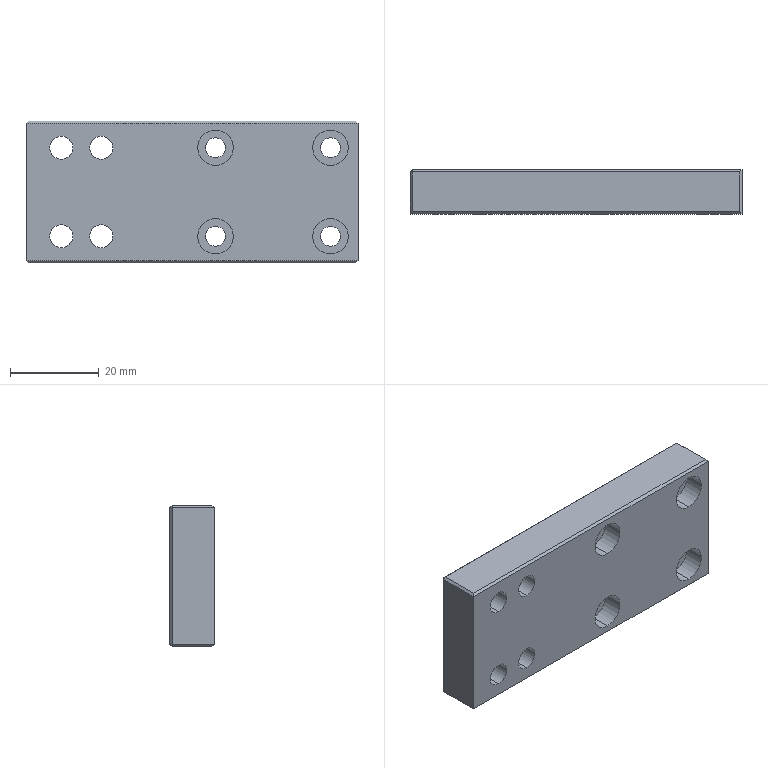Part | SolidWorks | features ICE 3, HoleWzd 2, Chamfer 1, Extrusion 1 | 1 solid | 61 faces | box 75 x 10 x 32 mm | volume 18437 mm3 | plane 31 | cylinder 30 | commonest cylinder face diameters 4.5 x8 5.2 x8 8 x8 10 x4 5 x2